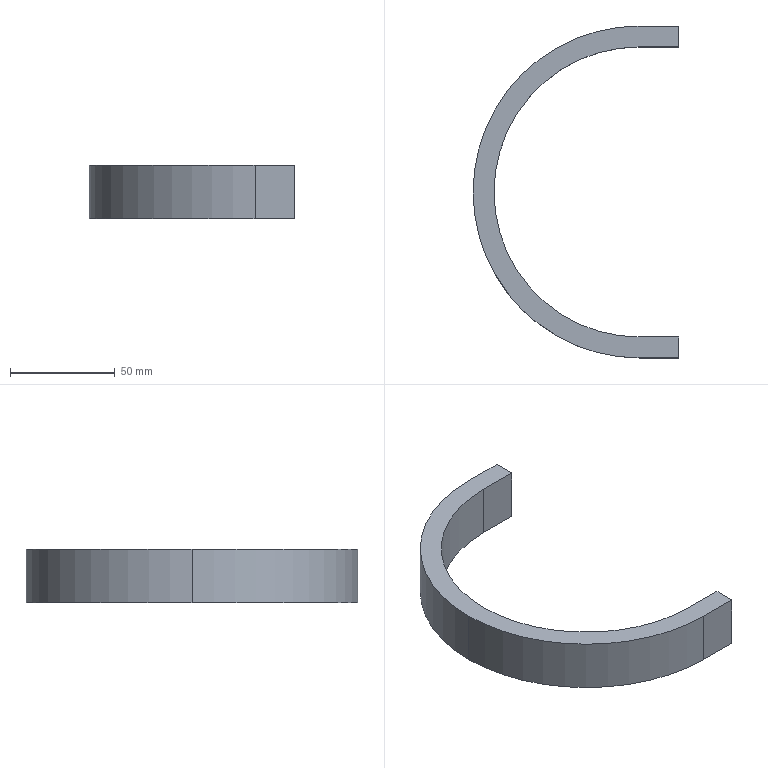Part | SolidWorks | features Extrusion 1 | 1 solid | 12 faces | box 98.425 x 158.75 x 25.4 mm | volume 69026 mm3 | plane 8 | cylinder 4 | commonest cylinder face diameters 138.75 x2 158.75 x2
STEP:
#1=CARTESIAN_POINT('',(-79.375,0.,12.7));
#2=VERTEX_POINT('',#1);
#3=CARTESIAN_POINT('',(0.,-79.375,12.7));
#4=VERTEX_POINT('',#3);
#5=CARTESIAN_POINT('',(0.,0.,12.7));
#6=DIRECTION('',(0.,0.,1.));
#7=DIRECTION('',(1.,0.,0.));
#8=AXIS2_PLACEMENT_3D('',#5,#6,#7);
#9=CIRCLE('',#8,79.375);
#10=EDGE_CURVE('',#2,#4,#9,.T.);
#11=ORIENTED_EDGE('',*,*,#10,.F.);
#12=CARTESIAN_POINT('',(-79.375,0.,-12.7));
#13=VERTEX_POINT('',#12);
#14=CARTESIAN_POINT('',(-79.375,0.,12.7));
#15=DIRECTION('',(0.,0.,-1.));
#16=VECTOR('',#15,1000.);
#17=LINE('',#14,#16);
#18=EDGE_CURVE('',#2,#13,#17,.T.);
#19=ORIENTED_EDGE('',*,*,#18,.T.);
#20=CARTESIAN_POINT('',(0.,-79.375,-12.7));
#21=VERTEX_POINT('',#20);
#22=CARTESIAN_POINT('',(0.,0.,-12.7));
#23=DIRECTION('',(0.,0.,1.));
#24=DIRECTION('',(1.,0.,0.));
#25=AXIS2_PLACEMENT_3D('',#22,#23,#24);
#26=CIRCLE('',#25,79.375);
#27=EDGE_CURVE('',#13,#21,#26,.T.);
#28=ORIENTED_EDGE('',*,*,#27,.T.);
#29=CARTESIAN_POINT('',(0.,-79.375,12.7));
#30=DIRECTION('',(0.,0.,-1.));
#31=VECTOR('',#30,1000.);
#32=LINE('',#29,#31);
#33=EDGE_CURVE('',#4,#21,#32,.T.);
#34=ORIENTED_EDGE('',*,*,#33,.F.);
#35=EDGE_LOOP('',(#11,#19,#28,#34));
#36=FACE_OUTER_BOUND('',#35,.T.);
#37=CARTESIAN_POINT('',(0.,0.,12.7));
#38=DIRECTION('',(0.,0.,-1.));
#39=DIRECTION('',(-1.,0.,0.));
#40=AXIS2_PLACEMENT_3D('',#37,#38,#39);
#41=CYLINDRICAL_SURFACE('',#40,79.375);
#42=ADVANCED_FACE('',(#36),#41,.T.);
#43=CARTESIAN_POINT('',(-69.375,0.,12.7));
#44=VERTEX_POINT('',#43);
#45=CARTESIAN_POINT('',(0.,69.375,12.7));
#46=VERTEX_POINT('',#45);
#47=CARTESIAN_POINT('',(0.,0.,12.7));
#48=DIRECTION('',(0.,0.,-1.));
#49=DIRECTION('',(1.,0.,0.));
#50=AXIS2_PLACEMENT_3D('',#47,#48,#49);
#51=CIRCLE('',#50,69.375);
#52=EDGE_CURVE('',#44,#46,#51,.T.);
#53=ORIENTED_EDGE('',*,*,#52,.F.);
#54=CARTESIAN_POINT('',(-69.375,0.,-12.7));
#55=VERTEX_POINT('',#54);
#56=CARTESIAN_POINT('',(-69.375,0.,12.7));
#57=DIRECTION('',(0.,0.,-1.));
#58=VECTOR('',#57,1000.);
#59=LINE('',#56,#58);
#60=EDGE_CURVE('',#44,#55,#59,.T.);
#61=ORIENTED_EDGE('',*,*,#60,.T.);
#62=CARTESIAN_POINT('',(0.,69.375,-12.7));
#63=VERTEX_POINT('',#62);
#64=CARTESIAN_POINT('',(0.,0.,-12.7));
#65=DIRECTION('',(0.,0.,-1.));
#66=DIRECTION('',(1.,0.,0.));
#67=AXIS2_PLACEMENT_3D('',#64,#65,#66);
#68=CIRCLE('',#67,69.375);
#69=EDGE_CURVE('',#55,#63,#68,.T.);
#70=ORIENTED_EDGE('',*,*,#69,.T.);
#71=CARTESIAN_POINT('',(0.,69.375,12.7));
#72=DIRECTION('',(0.,0.,-1.));
#73=VECTOR('',#72,1000.);
#74=LINE('',#71,#73);
#75=EDGE_CURVE('',#46,#63,#74,.T.);
#76=ORIENTED_EDGE('',*,*,#75,.F.);
#77=EDGE_LOOP('',(#53,#61,#70,#76));
#78=FACE_OUTER_BOUND('',#77,.T.);
#79=CARTESIAN_POINT('',(0.,0.,12.7));
#80=DIRECTION('',(0.,0.,-1.));
#81=DIRECTION('',(-1.,0.,0.));
#82=AXIS2_PLACEMENT_3D('',#79,#80,#81);
#83=CYLINDRICAL_SURFACE('',#82,69.375);
#84=ADVANCED_FACE('',(#78),#83,.F.);
#85=ORIENTED_EDGE('',*,*,#60,.F.);
#86=CARTESIAN_POINT('',(0.,-69.375,12.7));
#87=VERTEX_POINT('',#86);
#88=CARTESIAN_POINT('',(0.,0.,12.7));
#89=DIRECTION('',(0.,0.,-1.));
#90=DIRECTION('',(1.,0.,0.));
#91=AXIS2_PLACEMENT_3D('',#88,#89,#90);
#92=CIRCLE('',#91,69.375);
#93=EDGE_CURVE('',#87,#44,#92,.T.);
#94=ORIENTED_EDGE('',*,*,#93,.F.);
#95=CARTESIAN_POINT('',(0.,-69.375,-12.7));
#96=VERTEX_POINT('',#95);
#97=CARTESIAN_POINT('',(0.,-69.375,12.7));
#98=DIRECTION('',(0.,0.,-1.));
#99=VECTOR('',#98,1000.);
#100=LINE('',#97,#99);
#101=EDGE_CURVE('',#87,#96,#100,.T.);
#102=ORIENTED_EDGE('',*,*,#101,.T.);
#103=CARTESIAN_POINT('',(0.,0.,-12.7));
#104=DIRECTION('',(0.,0.,-1.));
#105=DIRECTION('',(1.,0.,0.));
#106=AXIS2_PLACEMENT_3D('',#103,#104,#105);
#107=CIRCLE('',#106,69.375);
#108=EDGE_CURVE('',#96,#55,#107,.T.);
#109=ORIENTED_EDGE('',*,*,#108,.T.);
#110=EDGE_LOOP('',(#85,#94,#102,#109));
#111=FACE_OUTER_BOUND('',#110,.T.);
#112=CARTESIAN_POINT('',(0.,0.,12.7));
#113=DIRECTION('',(0.,0.,-1.));
#114=DIRECTION('',(-1.,0.,0.));
#115=AXIS2_PLACEMENT_3D('',#112,#113,#114);
#116=CYLINDRICAL_SURFACE('',#115,69.375);
#117=ADVANCED_FACE('',(#111),#116,.F.);
#118=CARTESIAN_POINT('',(19.05,69.375,-12.7));
#119=VERTEX_POINT('',#118);
#120=CARTESIAN_POINT('',(0.,69.375,-12.7));
#121=DIRECTION('',(1.,0.,0.));
#122=VECTOR('',#121,1000.);
#123=LINE('',#120,#122);
#124=EDGE_CURVE('',#63,#119,#123,.T.);
#125=ORIENTED_EDGE('',*,*,#124,.T.);
#126=CARTESIAN_POINT('',(19.05,69.375,12.7));
#127=VERTEX_POINT('',#126);
#128=CARTESIAN_POINT('',(19.05,69.375,12.7));
#129=DIRECTION('',(0.,0.,-1.));
#130=VECTOR('',#129,1000.);
#131=LINE('',#128,#130);
#132=EDGE_CURVE('',#127,#119,#131,.T.);
#133=ORIENTED_EDGE('',*,*,#132,.F.);
#134=CARTESIAN_POINT('',(0.,69.375,12.7));
#135=DIRECTION('',(1.,0.,0.));
#136=VECTOR('',#135,1000.);
#137=LINE('',#134,#136);
#138=EDGE_CURVE('',#46,#127,#137,.T.);
#139=ORIENTED_EDGE('',*,*,#138,.F.);
#140=ORIENTED_EDGE('',*,*,#75,.T.);
#141=EDGE_LOOP('',(#125,#133,#139,#140));
#142=FACE_OUTER_BOUND('',#141,.T.);
#143=CARTESIAN_POINT('',(0.,69.375,12.7));
#144=DIRECTION('',(0.,1.,0.));
#145=DIRECTION('',(0.,0.,1.));
#146=AXIS2_PLACEMENT_3D('',#143,#144,#145);
#147=PLANE('',#146);
#148=ADVANCED_FACE('',(#142),#147,.F.);
#149=CARTESIAN_POINT('',(19.05,79.375,-12.7));
#150=VERTEX_POINT('',#149);
#151=CARTESIAN_POINT('',(19.05,79.375,-12.7));
#152=DIRECTION('',(0.,1.,0.));
#153=VECTOR('',#152,1000.);
#154=LINE('',#151,#153);
#155=EDGE_CURVE('',#119,#150,#154,.T.);
#156=ORIENTED_EDGE('',*,*,#155,.T.);
#157=CARTESIAN_POINT('',(19.05,79.375,12.7));
#158=VERTEX_POINT('',#157);
#159=CARTESIAN_POINT('',(19.05,79.375,12.7));
#160=DIRECTION('',(0.,0.,-1.));
#161=VECTOR('',#160,1000.);
#162=LINE('',#159,#161);
#163=EDGE_CURVE('',#158,#150,#162,.T.);
#164=ORIENTED_EDGE('',*,*,#163,.F.);
#165=CARTESIAN_POINT('',(19.05,79.375,12.7));
#166=DIRECTION('',(0.,1.,0.));
#167=VECTOR('',#166,1000.);
#168=LINE('',#165,#167);
#169=EDGE_CURVE('',#127,#158,#168,.T.);
#170=ORIENTED_EDGE('',*,*,#169,.F.);
#171=ORIENTED_EDGE('',*,*,#132,.T.);
#172=EDGE_LOOP('',(#156,#164,#170,#171));
#173=FACE_OUTER_BOUND('',#172,.T.);
#174=CARTESIAN_POINT('',(19.05,79.375,12.7));
#175=DIRECTION('',(-1.,0.,0.));
#176=DIRECTION('',(0.,0.,1.));
#177=AXIS2_PLACEMENT_3D('',#174,#175,#176);
#178=PLANE('',#177);
#179=ADVANCED_FACE('',(#173),#178,.F.);
#180=CARTESIAN_POINT('',(0.,79.375,-12.7));
#181=VERTEX_POINT('',#180);
#182=CARTESIAN_POINT('',(0.,79.375,-12.7));
#183=DIRECTION('',(-1.,0.,0.));
#184=VECTOR('',#183,1000.);
#185=LINE('',#182,#184);
#186=EDGE_CURVE('',#150,#181,#185,.T.);
#187=ORIENTED_EDGE('',*,*,#186,.T.);
#188=CARTESIAN_POINT('',(0.,79.375,12.7));
#189=VERTEX_POINT('',#188);
#190=CARTESIAN_POINT('',(0.,79.375,12.7));
#191=DIRECTION('',(0.,0.,-1.));
#192=VECTOR('',#191,1000.);
#193=LINE('',#190,#192);
#194=EDGE_CURVE('',#189,#181,#193,.T.);
#195=ORIENTED_EDGE('',*,*,#194,.F.);
#196=CARTESIAN_POINT('',(0.,79.375,12.7));
#197=DIRECTION('',(-1.,0.,0.));
#198=VECTOR('',#197,1000.);
#199=LINE('',#196,#198);
#200=EDGE_CURVE('',#158,#189,#199,.T.);
#201=ORIENTED_EDGE('',*,*,#200,.F.);
#202=ORIENTED_EDGE('',*,*,#163,.T.);
#203=EDGE_LOOP('',(#187,#195,#201,#202));
#204=FACE_OUTER_BOUND('',#203,.T.);
#205=CARTESIAN_POINT('',(0.,79.375,12.7));
#206=DIRECTION('',(0.,-1.,0.));
#207=DIRECTION('',(0.,0.,-1.));
#208=AXIS2_PLACEMENT_3D('',#205,#206,#207);
#209=PLANE('',#208);
#210=ADVANCED_FACE('',(#204),#209,.F.);
#211=ORIENTED_EDGE('',*,*,#18,.F.);
#212=CARTESIAN_POINT('',(0.,0.,12.7));
#213=DIRECTION('',(0.,0.,1.));
#214=DIRECTION('',(1.,0.,0.));
#215=AXIS2_PLACEMENT_3D('',#212,#213,#214);
#216=CIRCLE('',#215,79.375);
#217=EDGE_CURVE('',#189,#2,#216,.T.);
#218=ORIENTED_EDGE('',*,*,#217,.F.);
#219=ORIENTED_EDGE('',*,*,#194,.T.);
#220=CARTESIAN_POINT('',(0.,0.,-12.7));
#221=DIRECTION('',(0.,0.,1.));
#222=DIRECTION('',(1.,0.,0.));
#223=AXIS2_PLACEMENT_3D('',#220,#221,#222);
#224=CIRCLE('',#223,79.375);
#225=EDGE_CURVE('',#181,#13,#224,.T.);
#226=ORIENTED_EDGE('',*,*,#225,.T.);
#227=EDGE_LOOP('',(#211,#218,#219,#226));
#228=FACE_OUTER_BOUND('',#227,.T.);
#229=CARTESIAN_POINT('',(0.,0.,12.7));
#230=DIRECTION('',(0.,0.,-1.));
#231=DIRECTION('',(-1.,0.,0.));
#232=AXIS2_PLACEMENT_3D('',#229,#230,#231);
#233=CYLINDRICAL_SURFACE('',#232,79.375);
#234=ADVANCED_FACE('',(#228),#233,.T.);
#235=CARTESIAN_POINT('',(19.05,-79.375,-12.7));
#236=VERTEX_POINT('',#235);
#237=CARTESIAN_POINT('',(0.,-79.375,-12.7));
#238=DIRECTION('',(1.,0.,0.));
#239=VECTOR('',#238,1000.);
#240=LINE('',#237,#239);
#241=EDGE_CURVE('',#21,#236,#240,.T.);
#242=ORIENTED_EDGE('',*,*,#241,.T.);
#243=CARTESIAN_POINT('',(19.05,-79.375,12.7));
#244=VERTEX_POINT('',#243);
#245=CARTESIAN_POINT('',(19.05,-79.375,12.7));
#246=DIRECTION('',(0.,0.,-1.));
#247=VECTOR('',#246,1000.);
#248=LINE('',#245,#247);
#249=EDGE_CURVE('',#244,#236,#248,.T.);
#250=ORIENTED_EDGE('',*,*,#249,.F.);
#251=CARTESIAN_POINT('',(0.,-79.375,12.7));
#252=DIRECTION('',(1.,0.,0.));
#253=VECTOR('',#252,1000.);
#254=LINE('',#251,#253);
#255=EDGE_CURVE('',#4,#244,#254,.T.);
#256=ORIENTED_EDGE('',*,*,#255,.F.);
#257=ORIENTED_EDGE('',*,*,#33,.T.);
#258=EDGE_LOOP('',(#242,#250,#256,#257));
#259=FACE_OUTER_BOUND('',#258,.T.);
#260=CARTESIAN_POINT('',(0.,-79.375,12.7));
#261=DIRECTION('',(0.,1.,0.));
#262=DIRECTION('',(0.,0.,1.));
#263=AXIS2_PLACEMENT_3D('',#260,#261,#262);
#264=PLANE('',#263);
#265=ADVANCED_FACE('',(#259),#264,.F.);
#266=CARTESIAN_POINT('',(19.05,-69.375,-12.7));
#267=VERTEX_POINT('',#266);
#268=CARTESIAN_POINT('',(19.05,-69.375,-12.7));
#269=DIRECTION('',(0.,1.,0.));
#270=VECTOR('',#269,1000.);
#271=LINE('',#268,#270);
#272=EDGE_CURVE('',#236,#267,#271,.T.);
#273=ORIENTED_EDGE('',*,*,#272,.T.);
#274=CARTESIAN_POINT('',(19.05,-69.375,12.7));
#275=VERTEX_POINT('',#274);
#276=CARTESIAN_POINT('',(19.05,-69.375,12.7));
#277=DIRECTION('',(0.,0.,-1.));
#278=VECTOR('',#277,1000.);
#279=LINE('',#276,#278);
#280=EDGE_CURVE('',#275,#267,#279,.T.);
#281=ORIENTED_EDGE('',*,*,#280,.F.);
#282=CARTESIAN_POINT('',(19.05,-69.375,12.7));
#283=DIRECTION('',(0.,1.,0.));
#284=VECTOR('',#283,1000.);
#285=LINE('',#282,#284);
#286=EDGE_CURVE('',#244,#275,#285,.T.);
#287=ORIENTED_EDGE('',*,*,#286,.F.);
#288=ORIENTED_EDGE('',*,*,#249,.T.);
#289=EDGE_LOOP('',(#273,#281,#287,#288));
#290=FACE_OUTER_BOUND('',#289,.T.);
#291=CARTESIAN_POINT('',(19.05,-69.375,12.7));
#292=DIRECTION('',(-1.,0.,0.));
#293=DIRECTION('',(0.,0.,1.));
#294=AXIS2_PLACEMENT_3D('',#291,#292,#293);
#295=PLANE('',#294);
#296=ADVANCED_FACE('',(#290),#295,.F.);
#297=CARTESIAN_POINT('',(0.,-69.375,-12.7));
#298=DIRECTION('',(-1.,0.,0.));
#299=VECTOR('',#298,1000.);
#300=LINE('',#297,#299);
#301=EDGE_CURVE('',#267,#96,#300,.T.);
#302=ORIENTED_EDGE('',*,*,#301,.T.);
#303=ORIENTED_EDGE('',*,*,#101,.F.);
#304=CARTESIAN_POINT('',(0.,-69.375,12.7));
#305=DIRECTION('',(-1.,0.,0.));
#306=VECTOR('',#305,1000.);
#307=LINE('',#304,#306);
#308=EDGE_CURVE('',#275,#87,#307,.T.);
#309=ORIENTED_EDGE('',*,*,#308,.F.);
#310=ORIENTED_EDGE('',*,*,#280,.T.);
#311=EDGE_LOOP('',(#302,#303,#309,#310));
#312=FACE_OUTER_BOUND('',#311,.T.);
#313=CARTESIAN_POINT('',(0.,-69.375,12.7));
#314=DIRECTION('',(0.,-1.,0.));
#315=DIRECTION('',(0.,0.,-1.));
#316=AXIS2_PLACEMENT_3D('',#313,#314,#315);
#317=PLANE('',#316);
#318=ADVANCED_FACE('',(#312),#317,.F.);
#319=ORIENTED_EDGE('',*,*,#93,.T.);
#320=ORIENTED_EDGE('',*,*,#52,.T.);
#321=ORIENTED_EDGE('',*,*,#138,.T.);
#322=ORIENTED_EDGE('',*,*,#169,.T.);
#323=ORIENTED_EDGE('',*,*,#200,.T.);
#324=ORIENTED_EDGE('',*,*,#217,.T.);
#325=ORIENTED_EDGE('',*,*,#10,.T.);
#326=ORIENTED_EDGE('',*,*,#255,.T.);
#327=ORIENTED_EDGE('',*,*,#286,.T.);
#328=ORIENTED_EDGE('',*,*,#308,.T.);
#329=EDGE_LOOP('',(#319,#320,#321,#322,#323,#324,#325,#326,#327,#328));
#330=FACE_OUTER_BOUND('',#329,.T.);
#331=CARTESIAN_POINT('',(0.,0.,12.7));
#332=DIRECTION('',(0.,0.,1.));
#333=DIRECTION('',(1.,0.,0.));
#334=AXIS2_PLACEMENT_3D('',#331,#332,#333);
#335=PLANE('',#334);
#336=ADVANCED_FACE('',(#330),#335,.T.);
#337=ORIENTED_EDGE('',*,*,#108,.F.);
#338=ORIENTED_EDGE('',*,*,#301,.F.);
#339=ORIENTED_EDGE('',*,*,#272,.F.);
#340=ORIENTED_EDGE('',*,*,#241,.F.);
#341=ORIENTED_EDGE('',*,*,#27,.F.);
#342=ORIENTED_EDGE('',*,*,#225,.F.);
#343=ORIENTED_EDGE('',*,*,#186,.F.);
#344=ORIENTED_EDGE('',*,*,#155,.F.);
#345=ORIENTED_EDGE('',*,*,#124,.F.);
#346=ORIENTED_EDGE('',*,*,#69,.F.);
#347=EDGE_LOOP('',(#337,#338,#339,#340,#341,#342,#343,#344,#345,#346));
#348=FACE_OUTER_BOUND('',#347,.T.);
#349=CARTESIAN_POINT('',(0.,0.,-12.7));
#350=DIRECTION('',(0.,0.,1.));
#351=DIRECTION('',(1.,0.,0.));
#352=AXIS2_PLACEMENT_3D('',#349,#350,#351);
#353=PLANE('',#352);
#354=ADVANCED_FACE('',(#348),#353,.F.);
#355=CLOSED_SHELL('',(#42,#84,#117,#148,#179,#210,#234,#265,#296,#318,#336,#354));
#356=MANIFOLD_SOLID_BREP('',#355);
#357=CARTESIAN_POINT('',(0.,0.,0.));
#358=DIRECTION('',(0.,0.,1.));
#359=DIRECTION('',(1.,0.,0.));
#360=AXIS2_PLACEMENT_3D('',#357,#358,#359);
#361=(LENGTH_UNIT()NAMED_UNIT(*)SI_UNIT(.MILLI.,.METRE.));
#362=UNCERTAINTY_MEASURE_WITH_UNIT(LENGTH_MEASURE(0.00001),#361,'','');
#363=(NAMED_UNIT(*)PLANE_ANGLE_UNIT()SI_UNIT($,.RADIAN.));
#364=(NAMED_UNIT(*)SI_UNIT($,.STERADIAN.)SOLID_ANGLE_UNIT());
#365=(GEOMETRIC_REPRESENTATION_CONTEXT(3)GLOBAL_UNCERTAINTY_ASSIGNED_CONTEXT((#362))GLOBAL_UNIT_ASSIGNED_CONTEXT((#361,#363,#364))REPRESENTATION_CONTEXT('',''));
#366=ADVANCED_BREP_SHAPE_REPRESENTATION('',(#356,#360),#365);